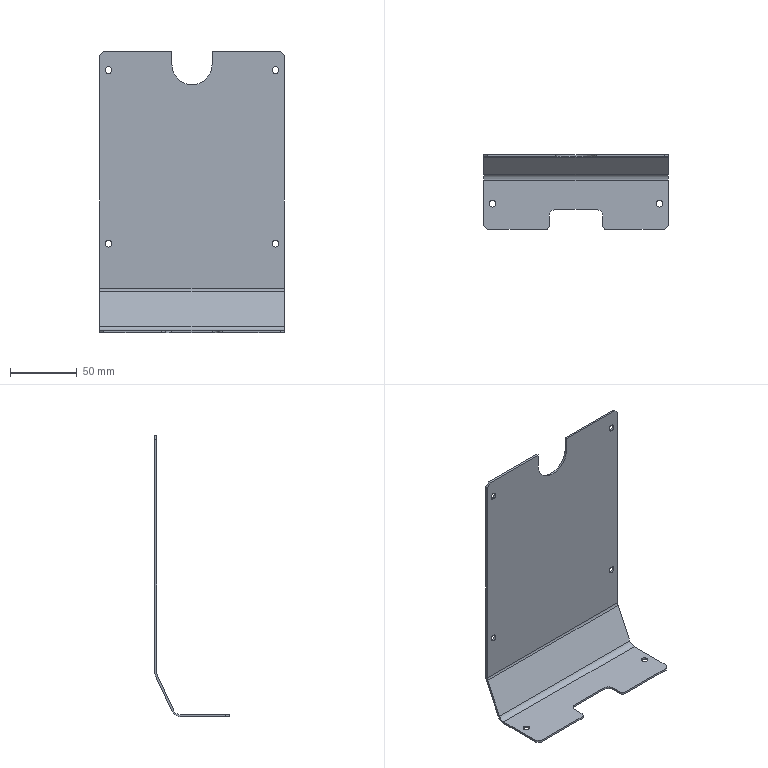Part | SolidWorks | features BaseBody 1 | 1 solid | 42 faces | box 138 x 55.773 x 210.513 mm | volume 50226 mm3 | cylinder 21 | plane 21 | commonest cylinder face diameters 5 x12 10 x4 6 x2 13 x2 30 x1
STEP:
#1=CARTESIAN_POINT('',(62.5,-33.973,-119.763));
#2=VERTEX_POINT('',#1);
#3=CARTESIAN_POINT('',(62.5,-38.973,-119.763));
#4=VERTEX_POINT('',#3);
#5=CARTESIAN_POINT('',(62.5,-36.473,-119.763));
#6=DIRECTION('',(0.,0.,1.));
#7=DIRECTION('',(0.,-1.,0.));
#8=AXIS2_PLACEMENT_3D('',#5,#6,#7);
#9=CIRCLE('',#8,2.5);
#10=EDGE_CURVE('',#2,#4,#9,.T.);
#11=ORIENTED_EDGE('',*,*,#10,.T.);
#12=CARTESIAN_POINT('',(62.5,-38.973,-121.263));
#13=VERTEX_POINT('',#12);
#14=CARTESIAN_POINT('',(62.5,-38.973,-121.263));
#15=DIRECTION('',(0.,0.,-1.));
#16=VECTOR('',#15,1000.);
#17=LINE('',#14,#16);
#18=EDGE_CURVE('',#4,#13,#17,.T.);
#19=ORIENTED_EDGE('',*,*,#18,.T.);
#20=CARTESIAN_POINT('',(62.5,-33.973,-121.263));
#21=VERTEX_POINT('',#20);
#22=CARTESIAN_POINT('',(62.5,-36.473,-121.263));
#23=DIRECTION('',(0.,0.,-1.));
#24=DIRECTION('',(0.,1.,0.));
#25=AXIS2_PLACEMENT_3D('',#22,#23,#24);
#26=CIRCLE('',#25,2.5);
#27=EDGE_CURVE('',#13,#21,#26,.T.);
#28=ORIENTED_EDGE('',*,*,#27,.T.);
#29=CARTESIAN_POINT('',(62.5,-33.973,-121.263));
#30=DIRECTION('',(0.,0.,-1.));
#31=VECTOR('',#30,1000.);
#32=LINE('',#29,#31);
#33=EDGE_CURVE('',#2,#21,#32,.T.);
#34=ORIENTED_EDGE('',*,*,#33,.F.);
#35=EDGE_LOOP('',(#11,#19,#28,#34));
#36=FACE_OUTER_BOUND('',#35,.T.);
#37=CARTESIAN_POINT('',(62.5,-36.473,-121.263));
#38=DIRECTION('',(0.,0.,-1.));
#39=DIRECTION('',(0.,1.,0.));
#40=AXIS2_PLACEMENT_3D('',#37,#38,#39);
#41=CYLINDRICAL_SURFACE('',#40,2.5);
#42=ADVANCED_FACE('',(#36),#41,.F.);
#43=CARTESIAN_POINT('',(-62.5,-33.973,-119.763));
#44=VERTEX_POINT('',#43);
#45=CARTESIAN_POINT('',(-62.5,-38.973,-119.763));
#46=VERTEX_POINT('',#45);
#47=CARTESIAN_POINT('',(-62.5,-36.473,-119.763));
#48=DIRECTION('',(0.,0.,1.));
#49=DIRECTION('',(0.,-1.,0.));
#50=AXIS2_PLACEMENT_3D('',#47,#48,#49);
#51=CIRCLE('',#50,2.5);
#52=EDGE_CURVE('',#44,#46,#51,.T.);
#53=ORIENTED_EDGE('',*,*,#52,.T.);
#54=CARTESIAN_POINT('',(-62.5,-38.973,-121.263));
#55=VERTEX_POINT('',#54);
#56=CARTESIAN_POINT('',(-62.5,-38.973,-121.263));
#57=DIRECTION('',(0.,0.,-1.));
#58=VECTOR('',#57,1000.);
#59=LINE('',#56,#58);
#60=EDGE_CURVE('',#46,#55,#59,.T.);
#61=ORIENTED_EDGE('',*,*,#60,.T.);
#62=CARTESIAN_POINT('',(-62.5,-33.973,-121.263));
#63=VERTEX_POINT('',#62);
#64=CARTESIAN_POINT('',(-62.5,-36.473,-121.263));
#65=DIRECTION('',(0.,0.,-1.));
#66=DIRECTION('',(0.,1.,0.));
#67=AXIS2_PLACEMENT_3D('',#64,#65,#66);
#68=CIRCLE('',#67,2.5);
#69=EDGE_CURVE('',#55,#63,#68,.T.);
#70=ORIENTED_EDGE('',*,*,#69,.T.);
#71=CARTESIAN_POINT('',(-62.5,-33.973,-121.263));
#72=DIRECTION('',(0.,0.,-1.));
#73=VECTOR('',#72,1000.);
#74=LINE('',#71,#73);
#75=EDGE_CURVE('',#44,#63,#74,.T.);
#76=ORIENTED_EDGE('',*,*,#75,.F.);
#77=EDGE_LOOP('',(#53,#61,#70,#76));
#78=FACE_OUTER_BOUND('',#77,.T.);
#79=CARTESIAN_POINT('',(-62.5,-36.473,-121.263));
#80=DIRECTION('',(0.,0.,-1.));
#81=DIRECTION('',(0.,1.,0.));
#82=AXIS2_PLACEMENT_3D('',#79,#80,#81);
#83=CYLINDRICAL_SURFACE('',#82,2.5);
#84=ADVANCED_FACE('',(#78),#83,.F.);
#85=CARTESIAN_POINT('',(62.5,-1.5,-57.25));
#86=VERTEX_POINT('',#85);
#87=CARTESIAN_POINT('',(62.5,-1.5,-52.25));
#88=VERTEX_POINT('',#87);
#89=CARTESIAN_POINT('',(62.5,-1.5,-54.75));
#90=DIRECTION('',(0.,1.,0.));
#91=DIRECTION('',(0.,0.,1.));
#92=AXIS2_PLACEMENT_3D('',#89,#90,#91);
#93=CIRCLE('',#92,2.5);
#94=EDGE_CURVE('',#86,#88,#93,.T.);
#95=ORIENTED_EDGE('',*,*,#94,.F.);
#96=CARTESIAN_POINT('',(62.5,0.,-57.25));
#97=VERTEX_POINT('',#96);
#98=CARTESIAN_POINT('',(62.5,0.,-57.25));
#99=DIRECTION('',(0.,1.,0.));
#100=VECTOR('',#99,1000.);
#101=LINE('',#98,#100);
#102=EDGE_CURVE('',#86,#97,#101,.T.);
#103=ORIENTED_EDGE('',*,*,#102,.T.);
#104=CARTESIAN_POINT('',(62.5,0.,-52.25));
#105=VERTEX_POINT('',#104);
#106=CARTESIAN_POINT('',(62.5,0.,-54.75));
#107=DIRECTION('',(0.,1.,0.));
#108=DIRECTION('',(0.,0.,1.));
#109=AXIS2_PLACEMENT_3D('',#106,#107,#108);
#110=CIRCLE('',#109,2.5);
#111=EDGE_CURVE('',#97,#105,#110,.T.);
#112=ORIENTED_EDGE('',*,*,#111,.T.);
#113=CARTESIAN_POINT('',(62.5,0.,-52.25));
#114=DIRECTION('',(0.,1.,0.));
#115=VECTOR('',#114,1000.);
#116=LINE('',#113,#115);
#117=EDGE_CURVE('',#88,#105,#116,.T.);
#118=ORIENTED_EDGE('',*,*,#117,.F.);
#119=EDGE_LOOP('',(#95,#103,#112,#118));
#120=FACE_OUTER_BOUND('',#119,.T.);
#121=CARTESIAN_POINT('',(62.5,0.,-54.75));
#122=DIRECTION('',(0.,1.,0.));
#123=DIRECTION('',(0.,0.,1.));
#124=AXIS2_PLACEMENT_3D('',#121,#122,#123);
#125=CYLINDRICAL_SURFACE('',#124,2.5);
#126=ADVANCED_FACE('',(#120),#125,.F.);
#127=CARTESIAN_POINT('',(-62.5,-1.5,-57.25));
#128=VERTEX_POINT('',#127);
#129=CARTESIAN_POINT('',(-62.5,-1.5,-52.25));
#130=VERTEX_POINT('',#129);
#131=CARTESIAN_POINT('',(-62.5,-1.5,-54.75));
#132=DIRECTION('',(0.,1.,0.));
#133=DIRECTION('',(0.,0.,1.));
#134=AXIS2_PLACEMENT_3D('',#131,#132,#133);
#135=CIRCLE('',#134,2.5);
#136=EDGE_CURVE('',#128,#130,#135,.T.);
#137=ORIENTED_EDGE('',*,*,#136,.F.);
#138=CARTESIAN_POINT('',(-62.5,0.,-57.25));
#139=VERTEX_POINT('',#138);
#140=CARTESIAN_POINT('',(-62.5,0.,-57.25));
#141=DIRECTION('',(0.,1.,0.));
#142=VECTOR('',#141,1000.);
#143=LINE('',#140,#142);
#144=EDGE_CURVE('',#128,#139,#143,.T.);
#145=ORIENTED_EDGE('',*,*,#144,.T.);
#146=CARTESIAN_POINT('',(-62.5,0.,-52.25));
#147=VERTEX_POINT('',#146);
#148=CARTESIAN_POINT('',(-62.5,0.,-54.75));
#149=DIRECTION('',(0.,1.,0.));
#150=DIRECTION('',(0.,0.,1.));
#151=AXIS2_PLACEMENT_3D('',#148,#149,#150);
#152=CIRCLE('',#151,2.5);
#153=EDGE_CURVE('',#139,#147,#152,.T.);
#154=ORIENTED_EDGE('',*,*,#153,.T.);
#155=CARTESIAN_POINT('',(-62.5,0.,-52.25));
#156=DIRECTION('',(0.,1.,0.));
#157=VECTOR('',#156,1000.);
#158=LINE('',#155,#157);
#159=EDGE_CURVE('',#130,#147,#158,.T.);
#160=ORIENTED_EDGE('',*,*,#159,.F.);
#161=EDGE_LOOP('',(#137,#145,#154,#160));
#162=FACE_OUTER_BOUND('',#161,.T.);
#163=CARTESIAN_POINT('',(-62.5,0.,-54.75));
#164=DIRECTION('',(0.,1.,0.));
#165=DIRECTION('',(0.,0.,1.));
#166=AXIS2_PLACEMENT_3D('',#163,#164,#165);
#167=CYLINDRICAL_SURFACE('',#166,2.5);
#168=ADVANCED_FACE('',(#162),#167,.F.);
#169=CARTESIAN_POINT('',(-62.5,-1.5,72.75));
#170=VERTEX_POINT('',#169);
#171=CARTESIAN_POINT('',(-62.5,-1.5,77.75));
#172=VERTEX_POINT('',#171);
#173=CARTESIAN_POINT('',(-62.5,-1.5,75.25));
#174=DIRECTION('',(0.,1.,0.));
#175=DIRECTION('',(0.,0.,1.));
#176=AXIS2_PLACEMENT_3D('',#173,#174,#175);
#177=CIRCLE('',#176,2.5);
#178=EDGE_CURVE('',#170,#172,#177,.T.);
#179=ORIENTED_EDGE('',*,*,#178,.F.);
#180=CARTESIAN_POINT('',(-62.5,0.,72.75));
#181=VERTEX_POINT('',#180);
#182=CARTESIAN_POINT('',(-62.5,0.,72.75));
#183=DIRECTION('',(0.,1.,0.));
#184=VECTOR('',#183,1000.);
#185=LINE('',#182,#184);
#186=EDGE_CURVE('',#170,#181,#185,.T.);
#187=ORIENTED_EDGE('',*,*,#186,.T.);
#188=CARTESIAN_POINT('',(-62.5,0.,77.75));
#189=VERTEX_POINT('',#188);
#190=CARTESIAN_POINT('',(-62.5,0.,75.25));
#191=DIRECTION('',(0.,1.,0.));
#192=DIRECTION('',(0.,0.,1.));
#193=AXIS2_PLACEMENT_3D('',#190,#191,#192);
#194=CIRCLE('',#193,2.5);
#195=EDGE_CURVE('',#181,#189,#194,.T.);
#196=ORIENTED_EDGE('',*,*,#195,.T.);
#197=CARTESIAN_POINT('',(-62.5,0.,77.75));
#198=DIRECTION('',(0.,1.,0.));
#199=VECTOR('',#198,1000.);
#200=LINE('',#197,#199);
#201=EDGE_CURVE('',#172,#189,#200,.T.);
#202=ORIENTED_EDGE('',*,*,#201,.F.);
#203=EDGE_LOOP('',(#179,#187,#196,#202));
#204=FACE_OUTER_BOUND('',#203,.T.);
#205=CARTESIAN_POINT('',(-62.5,0.,75.25));
#206=DIRECTION('',(0.,1.,0.));
#207=DIRECTION('',(0.,0.,1.));
#208=AXIS2_PLACEMENT_3D('',#205,#206,#207);
#209=CYLINDRICAL_SURFACE('',#208,2.5);
#210=ADVANCED_FACE('',(#204),#209,.F.);
#211=CARTESIAN_POINT('',(62.5,-1.5,72.75));
#212=VERTEX_POINT('',#211);
#213=CARTESIAN_POINT('',(62.5,-1.5,77.75));
#214=VERTEX_POINT('',#213);
#215=CARTESIAN_POINT('',(62.5,-1.5,75.25));
#216=DIRECTION('',(0.,1.,0.));
#217=DIRECTION('',(0.,0.,1.));
#218=AXIS2_PLACEMENT_3D('',#215,#216,#217);
#219=CIRCLE('',#218,2.5);
#220=EDGE_CURVE('',#212,#214,#219,.T.);
#221=ORIENTED_EDGE('',*,*,#220,.F.);
#222=CARTESIAN_POINT('',(62.5,0.,72.75));
#223=VERTEX_POINT('',#222);
#224=CARTESIAN_POINT('',(62.5,0.,72.75));
#225=DIRECTION('',(0.,1.,0.));
#226=VECTOR('',#225,1000.);
#227=LINE('',#224,#226);
#228=EDGE_CURVE('',#212,#223,#227,.T.);
#229=ORIENTED_EDGE('',*,*,#228,.T.);
#230=CARTESIAN_POINT('',(62.5,0.,77.75));
#231=VERTEX_POINT('',#230);
#232=CARTESIAN_POINT('',(62.5,0.,75.25));
#233=DIRECTION('',(0.,1.,0.));
#234=DIRECTION('',(0.,0.,1.));
#235=AXIS2_PLACEMENT_3D('',#232,#233,#234);
#236=CIRCLE('',#235,2.5);
#237=EDGE_CURVE('',#223,#231,#236,.T.);
#238=ORIENTED_EDGE('',*,*,#237,.T.);
#239=CARTESIAN_POINT('',(62.5,0.,77.75));
#240=DIRECTION('',(0.,1.,0.));
#241=VECTOR('',#240,1000.);
#242=LINE('',#239,#241);
#243=EDGE_CURVE('',#214,#231,#242,.T.);
#244=ORIENTED_EDGE('',*,*,#243,.F.);
#245=EDGE_LOOP('',(#221,#229,#238,#244));
#246=FACE_OUTER_BOUND('',#245,.T.);
#247=CARTESIAN_POINT('',(62.5,0.,75.25));
#248=DIRECTION('',(0.,1.,0.));
#249=DIRECTION('',(0.,0.,1.));
#250=AXIS2_PLACEMENT_3D('',#247,#248,#249);
#251=CYLINDRICAL_SURFACE('',#250,2.5);
#252=ADVANCED_FACE('',(#246),#251,.F.);
#253=CARTESIAN_POINT('',(-15.,-1.5,89.25));
#254=VERTEX_POINT('',#253);
#255=CARTESIAN_POINT('',(-15.,-1.5,79.25));
#256=VERTEX_POINT('',#255);
#257=CARTESIAN_POINT('',(-15.,-1.5,79.25));
#258=DIRECTION('',(0.,0.,-1.));
#259=VECTOR('',#258,1000.);
#260=LINE('',#257,#259);
#261=EDGE_CURVE('',#254,#256,#260,.T.);
#262=ORIENTED_EDGE('',*,*,#261,.T.);
#263=CARTESIAN_POINT('',(-15.,0.,79.25));
#264=VERTEX_POINT('',#263);
#265=CARTESIAN_POINT('',(-15.,-55.774,79.25));
#266=DIRECTION('',(0.,1.,0.));
#267=VECTOR('',#266,1000.);
#268=LINE('',#265,#267);
#269=EDGE_CURVE('',#256,#264,#268,.T.);
#270=ORIENTED_EDGE('',*,*,#269,.T.);
#271=CARTESIAN_POINT('',(-15.,0.,89.25));
#272=VERTEX_POINT('',#271);
#273=CARTESIAN_POINT('',(-15.,0.,79.25));
#274=DIRECTION('',(0.,0.,1.));
#275=VECTOR('',#274,1000.);
#276=LINE('',#273,#275);
#277=EDGE_CURVE('',#264,#272,#276,.T.);
#278=ORIENTED_EDGE('',*,*,#277,.T.);
#279=CARTESIAN_POINT('',(-15.,-55.774,89.25));
#280=DIRECTION('',(0.,1.,0.));
#281=VECTOR('',#280,1000.);
#282=LINE('',#279,#281);
#283=EDGE_CURVE('',#254,#272,#282,.T.);
#284=ORIENTED_EDGE('',*,*,#283,.F.);
#285=EDGE_LOOP('',(#262,#270,#278,#284));
#286=FACE_OUTER_BOUND('',#285,.T.);
#287=CARTESIAN_POINT('',(-15.,-55.774,79.25));
#288=DIRECTION('',(-1.,0.,0.));
#289=DIRECTION('',(0.,1.,0.));
#290=AXIS2_PLACEMENT_3D('',#287,#288,#289);
#291=PLANE('',#290);
#292=ADVANCED_FACE('',(#286),#291,.F.);
#293=CARTESIAN_POINT('',(15.,-1.5,79.25));
#294=VERTEX_POINT('',#293);
#295=CARTESIAN_POINT('',(15.,-1.5,89.25));
#296=VERTEX_POINT('',#295);
#297=CARTESIAN_POINT('',(15.,-1.5,79.25));
#298=DIRECTION('',(0.,0.,1.));
#299=VECTOR('',#298,1000.);
#300=LINE('',#297,#299);
#301=EDGE_CURVE('',#294,#296,#300,.T.);
#302=ORIENTED_EDGE('',*,*,#301,.T.);
#303=CARTESIAN_POINT('',(15.,0.,89.25));
#304=VERTEX_POINT('',#303);
#305=CARTESIAN_POINT('',(15.,-55.774,89.25));
#306=DIRECTION('',(0.,-1.,0.));
#307=VECTOR('',#306,1000.);
#308=LINE('',#305,#307);
#309=EDGE_CURVE('',#304,#296,#308,.T.);
#310=ORIENTED_EDGE('',*,*,#309,.F.);
#311=CARTESIAN_POINT('',(15.,0.,79.25));
#312=VERTEX_POINT('',#311);
#313=CARTESIAN_POINT('',(15.,0.,79.25));
#314=DIRECTION('',(0.,0.,-1.));
#315=VECTOR('',#314,1000.);
#316=LINE('',#313,#315);
#317=EDGE_CURVE('',#304,#312,#316,.T.);
#318=ORIENTED_EDGE('',*,*,#317,.T.);
#319=CARTESIAN_POINT('',(15.,-55.774,79.25));
#320=DIRECTION('',(0.,1.,0.));
#321=VECTOR('',#320,1000.);
#322=LINE('',#319,#321);
#323=EDGE_CURVE('',#294,#312,#322,.T.);
#324=ORIENTED_EDGE('',*,*,#323,.F.);
#325=EDGE_LOOP('',(#302,#310,#318,#324));
#326=FACE_OUTER_BOUND('',#325,.T.);
#327=CARTESIAN_POINT('',(15.,-55.774,79.25));
#328=DIRECTION('',(1.,0.,0.));
#329=DIRECTION('',(0.,0.,-1.));
#330=AXIS2_PLACEMENT_3D('',#327,#328,#329);
#331=PLANE('',#330);
#332=ADVANCED_FACE('',(#326),#331,.F.);
#333=CARTESIAN_POINT('',(0.,-1.5,79.25));
#334=DIRECTION('',(0.,-1.,0.));
#335=DIRECTION('',(0.,0.,1.));
#336=AXIS2_PLACEMENT_3D('',#333,#334,#335);
#337=CIRCLE('',#336,15.);
#338=EDGE_CURVE('',#256,#294,#337,.T.);
#339=ORIENTED_EDGE('',*,*,#338,.T.);
#340=ORIENTED_EDGE('',*,*,#323,.T.);
#341=CARTESIAN_POINT('',(0.,0.,79.25));
#342=DIRECTION('',(0.,1.,0.));
#343=DIRECTION('',(0.,0.,1.));
#344=AXIS2_PLACEMENT_3D('',#341,#342,#343);
#345=CIRCLE('',#344,15.);
#346=EDGE_CURVE('',#312,#264,#345,.T.);
#347=ORIENTED_EDGE('',*,*,#346,.T.);
#348=ORIENTED_EDGE('',*,*,#269,.F.);
#349=EDGE_LOOP('',(#339,#340,#347,#348));
#350=FACE_OUTER_BOUND('',#349,.T.);
#351=CARTESIAN_POINT('',(0.,-55.774,79.25));
#352=DIRECTION('',(0.,1.,0.));
#353=DIRECTION('',(0.,0.,1.));
#354=AXIS2_PLACEMENT_3D('',#351,#352,#353);
#355=CYLINDRICAL_SURFACE('',#354,15.);
#356=ADVANCED_FACE('',(#350),#355,.F.);
#357=CARTESIAN_POINT('',(20.,-52.773,-119.763));
#358=VERTEX_POINT('',#357);
#359=CARTESIAN_POINT('',(23.,-55.773,-119.763));
#360=VERTEX_POINT('',#359);
#361=CARTESIAN_POINT('',(23.,-52.773,-119.763));
#362=DIRECTION('',(0.,0.,1.));
#363=DIRECTION('',(0.,-1.,0.));
#364=AXIS2_PLACEMENT_3D('',#361,#362,#363);
#365=CIRCLE('',#364,3.);
#366=EDGE_CURVE('',#358,#360,#365,.T.);
#367=ORIENTED_EDGE('',*,*,#366,.F.);
#368=CARTESIAN_POINT('',(20.,-52.773,-121.263));
#369=VERTEX_POINT('',#368);
#370=CARTESIAN_POINT('',(20.,-52.773,89.251));
#371=DIRECTION('',(0.,0.,1.));
#372=VECTOR('',#371,1000.);
#373=LINE('',#370,#372);
#374=EDGE_CURVE('',#369,#358,#373,.T.);
#375=ORIENTED_EDGE('',*,*,#374,.F.);
#376=CARTESIAN_POINT('',(23.,-55.773,-121.263));
#377=VERTEX_POINT('',#376);
#378=CARTESIAN_POINT('',(23.,-52.773,-121.263));
#379=DIRECTION('',(0.,0.,-1.));
#380=DIRECTION('',(0.,-1.,0.));
#381=AXIS2_PLACEMENT_3D('',#378,#379,#380);
#382=CIRCLE('',#381,3.);
#383=EDGE_CURVE('',#377,#369,#382,.T.);
#384=ORIENTED_EDGE('',*,*,#383,.F.);
#385=CARTESIAN_POINT('',(23.,-55.773,-121.263));
#386=DIRECTION('',(0.,0.,-1.));
#387=VECTOR('',#386,1000.);
#388=LINE('',#385,#387);
#389=EDGE_CURVE('',#360,#377,#388,.T.);
#390=ORIENTED_EDGE('',*,*,#389,.F.);
#391=EDGE_LOOP('',(#367,#375,#384,#390));
#392=FACE_OUTER_BOUND('',#391,.T.);
#393=CARTESIAN_POINT('',(23.,-52.773,-121.263));
#394=DIRECTION('',(0.,0.,-1.));
#395=DIRECTION('',(0.,1.,0.));
#396=AXIS2_PLACEMENT_3D('',#393,#394,#395);
#397=CYLINDRICAL_SURFACE('',#396,3.);
#398=ADVANCED_FACE('',(#392),#397,.T.);
#399=CARTESIAN_POINT('',(-23.,-55.773,-119.763));
#400=VERTEX_POINT('',#399);
#401=CARTESIAN_POINT('',(-20.,-52.773,-119.763));
#402=VERTEX_POINT('',#401);
#403=CARTESIAN_POINT('',(-23.,-52.773,-119.763));
#404=DIRECTION('',(0.,0.,1.));
#405=DIRECTION('',(0.,-1.,0.));
#406=AXIS2_PLACEMENT_3D('',#403,#404,#405);
#407=CIRCLE('',#406,3.);
#408=EDGE_CURVE('',#400,#402,#407,.T.);
#409=ORIENTED_EDGE('',*,*,#408,.F.);
#410=CARTESIAN_POINT('',(-23.,-55.773,-121.263));
#411=VERTEX_POINT('',#410);
#412=CARTESIAN_POINT('',(-23.,-55.773,-121.263));
#413=DIRECTION('',(0.,0.,1.));
#414=VECTOR('',#413,1000.);
#415=LINE('',#412,#414);
#416=EDGE_CURVE('',#411,#400,#415,.T.);
#417=ORIENTED_EDGE('',*,*,#416,.F.);
#418=CARTESIAN_POINT('',(-20.,-52.773,-121.263));
#419=VERTEX_POINT('',#418);
#420=CARTESIAN_POINT('',(-23.,-52.773,-121.263));
#421=DIRECTION('',(0.,0.,-1.));
#422=DIRECTION('',(0.,-1.,0.));
#423=AXIS2_PLACEMENT_3D('',#420,#421,#422);
#424=CIRCLE('',#423,3.);
#425=EDGE_CURVE('',#419,#411,#424,.T.);
#426=ORIENTED_EDGE('',*,*,#425,.F.);
#427=CARTESIAN_POINT('',(-20.,-52.773,89.251));
#428=DIRECTION('',(0.,0.,-1.));
#429=VECTOR('',#428,1000.);
#430=LINE('',#427,#429);
#431=EDGE_CURVE('',#402,#419,#430,.T.);
#432=ORIENTED_EDGE('',*,*,#431,.F.);
#433=EDGE_LOOP('',(#409,#417,#426,#432));
#434=FACE_OUTER_BOUND('',#433,.T.);
#435=CARTESIAN_POINT('',(-23.,-52.773,89.251));
#436=DIRECTION('',(0.,0.,-1.));
#437=DIRECTION('',(0.,1.,0.));
#438=AXIS2_PLACEMENT_3D('',#435,#436,#437);
#439=CYLINDRICAL_SURFACE('',#438,3.);
#440=ADVANCED_FACE('',(#434),#439,.T.);
#441=CARTESIAN_POINT('',(15.,-40.773,-119.763));
#442=VERTEX_POINT('',#441);
#443=CARTESIAN_POINT('',(20.,-45.773,-119.763));
#444=VERTEX_POINT('',#443);
#445=CARTESIAN_POINT('',(15.,-45.773,-119.763));
#446=DIRECTION('',(0.,0.,-1.));
#447=DIRECTION('',(0.,-1.,0.));
#448=AXIS2_PLACEMENT_3D('',#445,#446,#447);
#449=CIRCLE('',#448,5.);
#450=EDGE_CURVE('',#442,#444,#449,.T.);
#451=ORIENTED_EDGE('',*,*,#450,.F.);
#452=CARTESIAN_POINT('',(15.,-40.773,-121.263));
#453=VERTEX_POINT('',#452);
#454=CARTESIAN_POINT('',(15.,-40.773,-119.763));
#455=DIRECTION('',(0.,0.,1.));
#456=VECTOR('',#455,1000.);
#457=LINE('',#454,#456);
#458=EDGE_CURVE('',#453,#442,#457,.T.);
#459=ORIENTED_EDGE('',*,*,#458,.F.);
#460=CARTESIAN_POINT('',(20.,-45.773,-121.263));
#461=VERTEX_POINT('',#460);
#462=CARTESIAN_POINT('',(15.,-45.773,-121.263));
#463=DIRECTION('',(0.,0.,1.));
#464=DIRECTION('',(0.,-1.,0.));
#465=AXIS2_PLACEMENT_3D('',#462,#463,#464);
#466=CIRCLE('',#465,5.);
#467=EDGE_CURVE('',#461,#453,#466,.T.);
#468=ORIENTED_EDGE('',*,*,#467,.F.);
#469=CARTESIAN_POINT('',(20.,-45.773,-121.263));
#470=DIRECTION('',(0.,0.,-1.));
#471=VECTOR('',#470,1000.);
#472=LINE('',#469,#471);
#473=EDGE_CURVE('',#444,#461,#472,.T.);
#474=ORIENTED_EDGE('',*,*,#473,.F.);
#475=EDGE_LOOP('',(#451,#459,#468,#474));
#476=FACE_OUTER_BOUND('',#475,.T.);
#477=CARTESIAN_POINT('',(15.,-45.773,89.251));
#478=DIRECTION('',(0.,0.,1.));
#479=DIRECTION('',(0.,-1.,0.));
#480=AXIS2_PLACEMENT_3D('',#477,#478,#479);
#481=CYLINDRICAL_SURFACE('',#480,5.);
#482=ADVANCED_FACE('',(#476),#481,.F.);
#483=CARTESIAN_POINT('',(-20.,-45.773,-119.763));
#484=VERTEX_POINT('',#483);
#485=CARTESIAN_POINT('',(-15.,-40.773,-119.763));
#486=VERTEX_POINT('',#485);
#487=CARTESIAN_POINT('',(-15.,-45.773,-119.763));
#488=DIRECTION('',(0.,0.,-1.));
#489=DIRECTION('',(0.,-1.,0.));
#490=AXIS2_PLACEMENT_3D('',#487,#488,#489);
#491=CIRCLE('',#490,5.);
#492=EDGE_CURVE('',#484,#486,#491,.T.);
#493=ORIENTED_EDGE('',*,*,#492,.F.);
#494=CARTESIAN_POINT('',(-20.,-45.773,-121.263));
#495=VERTEX_POINT('',#494);
#496=CARTESIAN_POINT('',(-20.,-45.773,-119.763));
#497=DIRECTION('',(0.,0.,1.));
#498=VECTOR('',#497,1000.);
#499=LINE('',#496,#498);
#500=EDGE_CURVE('',#495,#484,#499,.T.);
#501=ORIENTED_EDGE('',*,*,#500,.F.);
#502=CARTESIAN_POINT('',(-15.,-40.773,-121.263));
#503=VERTEX_POINT('',#502);
#504=CARTESIAN_POINT('',(-15.,-45.773,-121.263));
#505=DIRECTION('',(0.,0.,1.));
#506=DIRECTION('',(0.,-1.,0.));
#507=AXIS2_PLACEMENT_3D('',#504,#505,#506);
#508=CIRCLE('',#507,5.);
#509=EDGE_CURVE('',#503,#495,#508,.T.);
#510=ORIENTED_EDGE('',*,*,#509,.F.);
#511=CARTESIAN_POINT('',(-15.,-40.773,-121.263));
#512=DIRECTION('',(0.,0.,-1.));
#513=VECTOR('',#512,1000.);
#514=LINE('',#511,#513);
#515=EDGE_CURVE('',#486,#503,#514,.T.);
#516=ORIENTED_EDGE('',*,*,#515,.F.);
#517=EDGE_LOOP('',(#493,#501,#510,#516));
#518=FACE_OUTER_BOUND('',#517,.T.);
#519=CARTESIAN_POINT('',(-15.,-45.773,89.251));
#520=DIRECTION('',(0.,0.,1.));
#521=DIRECTION('',(0.,-1.,0.));
#522=AXIS2_PLACEMENT_3D('',#519,#520,#521);
#523=CYLINDRICAL_SURFACE('',#522,5.);
#524=ADVANCED_FACE('',(#518),#523,.F.);
#525=CARTESIAN_POINT('',(-20.,-55.773,-119.763));
#526=DIRECTION('',(0.,1.,0.));
#527=VECTOR('',#526,1000.);
#528=LINE('',#525,#527);
#529=EDGE_CURVE('',#402,#484,#528,.T.);
#530=ORIENTED_EDGE('',*,*,#529,.F.);
#531=ORIENTED_EDGE('',*,*,#431,.T.);
#532=CARTESIAN_POINT('',(-20.,-55.773,-121.263));
#533=DIRECTION('',(0.,1.,0.));
#534=VECTOR('',#533,1000.);
#535=LINE('',#532,#534);
#536=EDGE_CURVE('',#419,#495,#535,.T.);
#537=ORIENTED_EDGE('',*,*,#536,.T.);
#538=ORIENTED_EDGE('',*,*,#500,.T.);
#539=EDGE_LOOP('',(#530,#531,#537,#538));
#540=FACE_OUTER_BOUND('',#539,.T.);
#541=CARTESIAN_POINT('',(-20.,-55.773,89.251));
#542=DIRECTION('',(-1.,0.,0.));
#543=DIRECTION('',(0.,0.,1.));
#544=AXIS2_PLACEMENT_3D('',#541,#542,#543);
#545=PLANE('',#544);
#546=ADVANCED_FACE('',(#540),#545,.F.);
#547=CARTESIAN_POINT('',(20.,-40.773,-119.763));
#548=DIRECTION('',(1.,0.,0.));
#549=VECTOR('',#548,1000.);
#550=LINE('',#547,#549);
#551=EDGE_CURVE('',#486,#442,#550,.T.);
#552=ORIENTED_EDGE('',*,*,#551,.F.);
#553=ORIENTED_EDGE('',*,*,#515,.T.);
#554=CARTESIAN_POINT('',(20.,-40.773,-121.263));
#555=DIRECTION('',(1.,0.,0.));
#556=VECTOR('',#555,1000.);
#557=LINE('',#554,#556);
#558=EDGE_CURVE('',#503,#453,#557,.T.);
#559=ORIENTED_EDGE('',*,*,#558,.T.);
#560=ORIENTED_EDGE('',*,*,#458,.T.);
#561=EDGE_LOOP('',(#552,#553,#559,#560));
#562=FACE_OUTER_BOUND('',#561,.T.);
#563=CARTESIAN_POINT('',(20.,-40.773,89.251));
#564=DIRECTION('',(0.,1.,0.));
#565=DIRECTION('',(0.,0.,-1.));
#566=AXIS2_PLACEMENT_3D('',#563,#564,#565);
#567=PLANE('',#566);
#568=ADVANCED_FACE('',(#562),#567,.F.);
#569=CARTESIAN_POINT('',(20.,-55.773,-121.263));
#570=DIRECTION('',(0.,-1.,0.));
#571=VECTOR('',#570,1000.);
#572=LINE('',#569,#571);
#573=EDGE_CURVE('',#461,#369,#572,.T.);
#574=ORIENTED_EDGE('',*,*,#573,.T.);
#575=ORIENTED_EDGE('',*,*,#374,.T.);
#576=CARTESIAN_POINT('',(20.,-55.773,-119.763));
#577=DIRECTION('',(0.,-1.,0.));
#578=VECTOR('',#577,1000.);
#579=LINE('',#576,#578);
#580=EDGE_CURVE('',#444,#358,#579,.T.);
#581=ORIENTED_EDGE('',*,*,#580,.F.);
#582=ORIENTED_EDGE('',*,*,#473,.T.);
#583=EDGE_LOOP('',(#574,#575,#581,#582));
#584=FACE_OUTER_BOUND('',#583,.T.);
#585=CARTESIAN_POINT('',(20.,-55.773,89.251));
#586=DIRECTION('',(1.,0.,0.));
#587=DIRECTION('',(0.,1.,0.));
#588=AXIS2_PLACEMENT_3D('',#585,#586,#587);
#589=PLANE('',#588);
#590=ADVANCED_FACE('',(#584),#589,.F.);
#591=CARTESIAN_POINT('',(69.,-52.773,-121.263));
#592=VERTEX_POINT('',#591);
#593=CARTESIAN_POINT('',(66.,-55.773,-121.263));
#594=VERTEX_POINT('',#593);
#595=CARTESIAN_POINT('',(66.,-55.773,-121.263));
#596=DIRECTION('',(-0.7071,-0.7071,0.));
#597=VECTOR('',#596,1000.);
#598=LINE('',#595,#597);
#599=EDGE_CURVE('',#592,#594,#598,.T.);
#600=ORIENTED_EDGE('',*,*,#599,.F.);
#601=CARTESIAN_POINT('',(69.,-52.773,-119.763));
#602=VERTEX_POINT('',#601);
#603=CARTESIAN_POINT('',(69.,-52.773,-121.263));
#604=DIRECTION('',(0.,0.,-1.));
#605=VECTOR('',#604,1000.);
#606=LINE('',#603,#605);
#607=EDGE_CURVE('',#602,#592,#606,.T.);
#608=ORIENTED_EDGE('',*,*,#607,.F.);
#609=CARTESIAN_POINT('',(66.,-55.773,-119.763));
#610=VERTEX_POINT('',#609);
#611=CARTESIAN_POINT('',(60.886,-60.886,-119.763));
#612=DIRECTION('',(0.7071,0.7071,0.));
#613=VECTOR('',#612,1000.);
#614=LINE('',#611,#613);
#615=EDGE_CURVE('',#610,#602,#614,.T.);
#616=ORIENTED_EDGE('',*,*,#615,.F.);
#617=CARTESIAN_POINT('',(66.,-55.773,-121.263));
#618=DIRECTION('',(0.,0.,1.));
#619=VECTOR('',#618,1000.);
#620=LINE('',#617,#619);
#621=EDGE_CURVE('',#594,#610,#620,.T.);
#622=ORIENTED_EDGE('',*,*,#621,.F.);
#623=EDGE_LOOP('',(#600,#608,#616,#622));
#624=FACE_OUTER_BOUND('',#623,.T.);
#625=CARTESIAN_POINT('',(66.,-55.773,-121.263));
#626=DIRECTION('',(-0.7071,0.7071,0.));
#627=DIRECTION('',(0.,0.,1.));
#628=AXIS2_PLACEMENT_3D('',#625,#626,#627);
#629=PLANE('',#628);
#630=ADVANCED_FACE('',(#624),#629,.F.);
#631=CARTESIAN_POINT('',(69.,-1.5,86.25));
#632=VERTEX_POINT('',#631);
#633=CARTESIAN_POINT('',(66.,-1.5,89.25));
#634=VERTEX_POINT('',#633);
#635=CARTESIAN_POINT('',(66.,-1.5,89.25));
#636=DIRECTION('',(-0.7071,0.,0.7071));
#637=VECTOR('',#636,1000.);
#638=LINE('',#635,#637);
#639=EDGE_CURVE('',#632,#634,#638,.T.);
#640=ORIENTED_EDGE('',*,*,#639,.F.);
#641=CARTESIAN_POINT('',(69.,0.,86.25));
#642=VERTEX_POINT('',#641);
#643=CARTESIAN_POINT('',(69.,-1.5,86.25));
#644=DIRECTION('',(0.,-1.,0.));
#645=VECTOR('',#644,1000.);
#646=LINE('',#643,#645);
#647=EDGE_CURVE('',#642,#632,#646,.T.);
#648=ORIENTED_EDGE('',*,*,#647,.F.);
#649=CARTESIAN_POINT('',(66.,0.,89.25));
#650=VERTEX_POINT('',#649);
#651=CARTESIAN_POINT('',(77.625,0.,77.625));
#652=DIRECTION('',(0.7071,0.,-0.7071));
#653=VECTOR('',#652,1000.);
#654=LINE('',#651,#653);
#655=EDGE_CURVE('',#650,#642,#654,.T.);
#656=ORIENTED_EDGE('',*,*,#655,.F.);
#657=CARTESIAN_POINT('',(66.,-1.5,89.25));
#658=DIRECTION('',(0.,1.,0.));
#659=VECTOR('',#658,1000.);
#660=LINE('',#657,#659);
#661=EDGE_CURVE('',#634,#650,#660,.T.);
#662=ORIENTED_EDGE('',*,*,#661,.F.);
#663=EDGE_LOOP('',(#640,#648,#656,#662));
#664=FACE_OUTER_BOUND('',#663,.T.);
#665=CARTESIAN_POINT('',(66.,-1.5,89.25));
#666=DIRECTION('',(-0.7071,0.,-0.7071));
#667=DIRECTION('',(-0.7071,0.,0.7071));
#668=AXIS2_PLACEMENT_3D('',#665,#666,#667);
#669=PLANE('',#668);
#670=ADVANCED_FACE('',(#664),#669,.F.);
#671=CARTESIAN_POINT('',(-66.,-1.5,89.25));
#672=VERTEX_POINT('',#671);
#673=CARTESIAN_POINT('',(-69.,-1.5,86.25));
#674=VERTEX_POINT('',#673);
#675=CARTESIAN_POINT('',(-69.,-1.5,86.25));
#676=DIRECTION('',(-0.7071,0.,-0.7071));
#677=VECTOR('',#676,1000.);
#678=LINE('',#675,#677);
#679=EDGE_CURVE('',#672,#674,#678,.T.);
#680=ORIENTED_EDGE('',*,*,#679,.F.);
#681=CARTESIAN_POINT('',(-66.,0.,89.25));
#682=VERTEX_POINT('',#681);
#683=CARTESIAN_POINT('',(-66.,-1.5,89.25));
#684=DIRECTION('',(0.,-1.,0.));
#685=VECTOR('',#684,1000.);
#686=LINE('',#683,#685);
#687=EDGE_CURVE('',#682,#672,#686,.T.);
#688=ORIENTED_EDGE('',*,*,#687,.F.);
#689=CARTESIAN_POINT('',(-69.,0.,86.25));
#690=VERTEX_POINT('',#689);
#691=CARTESIAN_POINT('',(-77.625,0.,77.625));
#692=DIRECTION('',(0.7071,0.,0.7071));
#693=VECTOR('',#692,1000.);
#694=LINE('',#691,#693);
#695=EDGE_CURVE('',#690,#682,#694,.T.);
#696=ORIENTED_EDGE('',*,*,#695,.F.);
#697=CARTESIAN_POINT('',(-69.,-1.5,86.25));
#698=DIRECTION('',(0.,1.,0.));
#699=VECTOR('',#698,1000.);
#700=LINE('',#697,#699);
#701=EDGE_CURVE('',#674,#690,#700,.T.);
#702=ORIENTED_EDGE('',*,*,#701,.F.);
#703=EDGE_LOOP('',(#680,#688,#696,#702));
#704=FACE_OUTER_BOUND('',#703,.T.);
#705=CARTESIAN_POINT('',(-69.,-1.5,86.25));
#706=DIRECTION('',(0.7071,0.,-0.7071));
#707=DIRECTION('',(0.,-1.,0.));
#708=AXIS2_PLACEMENT_3D('',#705,#706,#707);
#709=PLANE('',#708);
#710=ADVANCED_FACE('',(#704),#709,.F.);
#711=CARTESIAN_POINT('',(-66.,-55.773,-121.263));
#712=VERTEX_POINT('',#711);
#713=CARTESIAN_POINT('',(-69.,-52.773,-121.263));
#714=VERTEX_POINT('',#713);
#715=CARTESIAN_POINT('',(-69.,-52.773,-121.263));
#716=DIRECTION('',(-0.7071,0.7071,0.));
#717=VECTOR('',#716,1000.);
#718=LINE('',#715,#717);
#719=EDGE_CURVE('',#712,#714,#718,.T.);
#720=ORIENTED_EDGE('',*,*,#719,.F.);
#721=CARTESIAN_POINT('',(-66.,-55.773,-119.763));
#722=VERTEX_POINT('',#721);
#723=CARTESIAN_POINT('',(-66.,-55.773,-121.263));
#724=DIRECTION('',(0.,0.,-1.));
#725=VECTOR('',#724,1000.);
#726=LINE('',#723,#725);
#727=EDGE_CURVE('',#722,#712,#726,.T.);
#728=ORIENTED_EDGE('',*,*,#727,.F.);
#729=CARTESIAN_POINT('',(-69.,-52.773,-119.763));
#730=VERTEX_POINT('',#729);
#731=CARTESIAN_POINT('',(-60.886,-60.886,-119.763));
#732=DIRECTION('',(0.7071,-0.7071,0.));
#733=VECTOR('',#732,1000.);
#734=LINE('',#731,#733);
#735=EDGE_CURVE('',#730,#722,#734,.T.);
#736=ORIENTED_EDGE('',*,*,#735,.F.);
#737=CARTESIAN_POINT('',(-69.,-52.773,-121.263));
#738=DIRECTION('',(0.,0.,1.));
#739=VECTOR('',#738,1000.);
#740=LINE('',#737,#739);
#741=EDGE_CURVE('',#714,#730,#740,.T.);
#742=ORIENTED_EDGE('',*,*,#741,.F.);
#743=EDGE_LOOP('',(#720,#728,#736,#742));
#744=FACE_OUTER_BOUND('',#743,.T.);
#745=CARTESIAN_POINT('',(-69.,-52.773,-121.263));
#746=DIRECTION('',(0.7071,0.7071,0.));
#747=DIRECTION('',(0.,0.,-1.));
#748=AXIS2_PLACEMENT_3D('',#745,#746,#747);
#749=PLANE('',#748);
#750=ADVANCED_FACE('',(#744),#749,.F.);
#751=CARTESIAN_POINT('',(-69.,-55.773,-121.263));
#752=DIRECTION('',(-1.,0.,0.));
#753=VECTOR('',#752,1000.);
#754=LINE('',#751,#753);
#755=EDGE_CURVE('',#411,#712,#754,.T.);
#756=ORIENTED_EDGE('',*,*,#755,.F.);
#757=ORIENTED_EDGE('',*,*,#416,.T.);
#758=CARTESIAN_POINT('',(-69.,-55.773,-119.763));
#759=DIRECTION('',(-1.,0.,0.));
#760=VECTOR('',#759,1000.);
#761=LINE('',#758,#760);
#762=EDGE_CURVE('',#400,#722,#761,.T.);
#763=ORIENTED_EDGE('',*,*,#762,.T.);
#764=ORIENTED_EDGE('',*,*,#727,.T.);
#765=EDGE_LOOP('',(#756,#757,#763,#764));
#766=FACE_OUTER_BOUND('',#765,.T.);
#767=CARTESIAN_POINT('',(-69.,-55.773,-121.263));
#768=DIRECTION('',(0.,1.,0.));
#769=DIRECTION('',(0.,0.,-1.));
#770=AXIS2_PLACEMENT_3D('',#767,#768,#769);
#771=PLANE('',#770);
#772=ADVANCED_FACE('',(#766),#771,.F.);
#773=ORIENTED_EDGE('',*,*,#52,.F.);
#774=CARTESIAN_POINT('',(-62.5,-36.473,-119.763));
#775=DIRECTION('',(0.,0.,1.));
#776=DIRECTION('',(0.,-1.,0.));
#777=AXIS2_PLACEMENT_3D('',#774,#775,#776);
#778=CIRCLE('',#777,2.5);
#779=EDGE_CURVE('',#46,#44,#778,.T.);
#780=ORIENTED_EDGE('',*,*,#779,.F.);
#781=EDGE_LOOP('',(#773,#780));
#782=FACE_BOUND('',#781,.T.);
#783=ORIENTED_EDGE('',*,*,#10,.F.);
#784=CARTESIAN_POINT('',(62.5,-36.473,-119.763));
#785=DIRECTION('',(0.,0.,1.));
#786=DIRECTION('',(0.,-1.,0.));
#787=AXIS2_PLACEMENT_3D('',#784,#785,#786);
#788=CIRCLE('',#787,2.5);
#789=EDGE_CURVE('',#4,#2,#788,.T.);
#790=ORIENTED_EDGE('',*,*,#789,.F.);
#791=EDGE_LOOP('',(#783,#790));
#792=FACE_BOUND('',#791,.T.);
#793=ORIENTED_EDGE('',*,*,#762,.F.);
#794=ORIENTED_EDGE('',*,*,#408,.T.);
#795=ORIENTED_EDGE('',*,*,#529,.T.);
#796=ORIENTED_EDGE('',*,*,#492,.T.);
#797=ORIENTED_EDGE('',*,*,#551,.T.);
#798=ORIENTED_EDGE('',*,*,#450,.T.);
#799=ORIENTED_EDGE('',*,*,#580,.T.);
#800=ORIENTED_EDGE('',*,*,#366,.T.);
#801=CARTESIAN_POINT('',(-69.,-55.773,-119.763));
#802=DIRECTION('',(-1.,0.,0.));
#803=VECTOR('',#802,1000.);
#804=LINE('',#801,#803);
#805=EDGE_CURVE('',#610,#360,#804,.T.);
#806=ORIENTED_EDGE('',*,*,#805,.F.);
#807=ORIENTED_EDGE('',*,*,#615,.T.);
#808=CARTESIAN_POINT('',(69.,-18.914,-119.763));
#809=VERTEX_POINT('',#808);
#810=CARTESIAN_POINT('',(69.,-55.773,-119.763));
#811=DIRECTION('',(0.,-1.,0.));
#812=VECTOR('',#811,1000.);
#813=LINE('',#810,#812);
#814=EDGE_CURVE('',#809,#602,#813,.T.);
#815=ORIENTED_EDGE('',*,*,#814,.F.);
#816=CARTESIAN_POINT('',(-69.,-18.914,-119.763));
#817=VERTEX_POINT('',#816);
#818=CARTESIAN_POINT('',(-69.,-18.914,-119.763));
#819=DIRECTION('',(1.,0.,0.));
#820=VECTOR('',#819,1000.);
#821=LINE('',#818,#820);
#822=EDGE_CURVE('',#817,#809,#821,.T.);
#823=ORIENTED_EDGE('',*,*,#822,.F.);
#824=CARTESIAN_POINT('',(-69.,-15.728,-119.763));
#825=DIRECTION('',(0.,1.,0.));
#826=VECTOR('',#825,1000.);
#827=LINE('',#824,#826);
#828=EDGE_CURVE('',#730,#817,#827,.T.);
#829=ORIENTED_EDGE('',*,*,#828,.F.);
#830=ORIENTED_EDGE('',*,*,#735,.T.);
#831=EDGE_LOOP('',(#793,#794,#795,#796,#797,#798,#799,#800,#806,#807,#815,#823,#829,#830));
#832=FACE_OUTER_BOUND('',#831,.T.);
#833=CARTESIAN_POINT('',(0.,0.,-119.763));
#834=DIRECTION('',(0.,0.,1.));
#835=DIRECTION('',(0.,-1.,0.));
#836=AXIS2_PLACEMENT_3D('',#833,#834,#835);
#837=PLANE('',#836);
#838=ADVANCED_FACE('',(#782,#792,#832),#837,.T.);
#839=CARTESIAN_POINT('',(-62.5,-36.473,-121.263));
#840=DIRECTION('',(0.,0.,-1.));
#841=DIRECTION('',(0.,1.,0.));
#842=AXIS2_PLACEMENT_3D('',#839,#840,#841);
#843=CIRCLE('',#842,2.5);
#844=EDGE_CURVE('',#63,#55,#843,.T.);
#845=ORIENTED_EDGE('',*,*,#844,.F.);
#846=ORIENTED_EDGE('',*,*,#69,.F.);
#847=EDGE_LOOP('',(#845,#846));
#848=FACE_BOUND('',#847,.T.);
#849=CARTESIAN_POINT('',(62.5,-36.473,-121.263));
#850=DIRECTION('',(0.,0.,-1.));
#851=DIRECTION('',(0.,1.,0.));
#852=AXIS2_PLACEMENT_3D('',#849,#850,#851);
#853=CIRCLE('',#852,2.5);
#854=EDGE_CURVE('',#21,#13,#853,.T.);
#855=ORIENTED_EDGE('',*,*,#854,.F.);
#856=ORIENTED_EDGE('',*,*,#27,.F.);
#857=EDGE_LOOP('',(#855,#856));
#858=FACE_BOUND('',#857,.T.);
#859=ORIENTED_EDGE('',*,*,#536,.F.);
#860=ORIENTED_EDGE('',*,*,#425,.T.);
#861=ORIENTED_EDGE('',*,*,#755,.T.);
#862=ORIENTED_EDGE('',*,*,#719,.T.);
#863=CARTESIAN_POINT('',(-69.,-18.914,-121.263));
#864=VERTEX_POINT('',#863);
#865=CARTESIAN_POINT('',(-69.,-15.728,-121.263));
#866=DIRECTION('',(0.,1.,0.));
#867=VECTOR('',#866,1000.);
#868=LINE('',#865,#867);
#869=EDGE_CURVE('',#714,#864,#868,.T.);
#870=ORIENTED_EDGE('',*,*,#869,.T.);
#871=CARTESIAN_POINT('',(69.,-18.914,-121.263));
#872=VERTEX_POINT('',#871);
#873=CARTESIAN_POINT('',(0.,-18.914,-121.263));
#874=DIRECTION('',(-1.,0.,0.));
#875=VECTOR('',#874,1000.);
#876=LINE('',#873,#875);
#877=EDGE_CURVE('',#872,#864,#876,.T.);
#878=ORIENTED_EDGE('',*,*,#877,.F.);
#879=CARTESIAN_POINT('',(69.,-55.773,-121.263));
#880=DIRECTION('',(0.,-1.,0.));
#881=VECTOR('',#880,1000.);
#882=LINE('',#879,#881);
#883=EDGE_CURVE('',#872,#592,#882,.T.);
#884=ORIENTED_EDGE('',*,*,#883,.T.);
#885=ORIENTED_EDGE('',*,*,#599,.T.);
#886=CARTESIAN_POINT('',(-69.,-55.773,-121.263));
#887=DIRECTION('',(-1.,0.,0.));
#888=VECTOR('',#887,1000.);
#889=LINE('',#886,#888);
#890=EDGE_CURVE('',#594,#377,#889,.T.);
#891=ORIENTED_EDGE('',*,*,#890,.T.);
#892=ORIENTED_EDGE('',*,*,#383,.T.);
#893=ORIENTED_EDGE('',*,*,#573,.F.);
#894=ORIENTED_EDGE('',*,*,#467,.T.);
#895=ORIENTED_EDGE('',*,*,#558,.F.);
#896=ORIENTED_EDGE('',*,*,#509,.T.);
#897=EDGE_LOOP('',(#859,#860,#861,#862,#870,#878,#884,#885,#891,#892,#893,#894,#895,#896));
#898=FACE_OUTER_BOUND('',#897,.T.);
#899=CARTESIAN_POINT('',(0.,0.,-121.263));
#900=DIRECTION('',(0.,0.,1.));
#901=DIRECTION('',(0.,-1.,0.));
#902=AXIS2_PLACEMENT_3D('',#899,#900,#901);
#903=PLANE('',#902);
#904=ADVANCED_FACE('',(#848,#858,#898),#903,.F.);
#905=CARTESIAN_POINT('',(69.,-14.382,-116.876));
#906=VERTEX_POINT('',#905);
#907=CARTESIAN_POINT('',(-69.,-14.382,-116.876));
#908=VERTEX_POINT('',#907);
#909=CARTESIAN_POINT('',(69.,-14.382,-116.876));
#910=DIRECTION('',(-1.,0.,0.));
#911=VECTOR('',#910,1000.);
#912=LINE('',#909,#911);
#913=EDGE_CURVE('',#906,#908,#912,.T.);
#914=ORIENTED_EDGE('',*,*,#913,.T.);
#915=CARTESIAN_POINT('',(-69.,-18.914,-114.763));
#916=DIRECTION('',(-1.,0.,0.));
#917=DIRECTION('',(0.,0.,-1.));
#918=AXIS2_PLACEMENT_3D('',#915,#916,#917);
#919=CIRCLE('',#918,5.);
#920=EDGE_CURVE('',#908,#817,#919,.T.);
#921=ORIENTED_EDGE('',*,*,#920,.T.);
#922=ORIENTED_EDGE('',*,*,#822,.T.);
#923=CARTESIAN_POINT('',(69.,-18.914,-114.763));
#924=DIRECTION('',(1.,0.,0.));
#925=DIRECTION('',(0.,0.,-1.));
#926=AXIS2_PLACEMENT_3D('',#923,#924,#925);
#927=CIRCLE('',#926,5.);
#928=EDGE_CURVE('',#809,#906,#927,.T.);
#929=ORIENTED_EDGE('',*,*,#928,.T.);
#930=EDGE_LOOP('',(#914,#921,#922,#929));
#931=FACE_OUTER_BOUND('',#930,.T.);
#932=CARTESIAN_POINT('',(69.,-18.914,-114.763));
#933=DIRECTION('',(1.,0.,0.));
#934=DIRECTION('',(0.,0.,-1.));
#935=AXIS2_PLACEMENT_3D('',#932,#933,#934);
#936=CYLINDRICAL_SURFACE('',#935,5.);
#937=ADVANCED_FACE('',(#931),#936,.F.);
#938=CARTESIAN_POINT('',(69.,-13.023,-117.51));
#939=VERTEX_POINT('',#938);
#940=CARTESIAN_POINT('',(-69.,-13.023,-117.51));
#941=VERTEX_POINT('',#940);
#942=CARTESIAN_POINT('',(69.,-13.023,-117.51));
#943=DIRECTION('',(-1.,0.,0.));
#944=VECTOR('',#943,1000.);
#945=LINE('',#942,#944);
#946=EDGE_CURVE('',#939,#941,#945,.T.);
#947=ORIENTED_EDGE('',*,*,#946,.F.);
#948=CARTESIAN_POINT('',(69.,-18.914,-114.763));
#949=DIRECTION('',(1.,0.,0.));
#950=DIRECTION('',(0.,0.,-1.));
#951=AXIS2_PLACEMENT_3D('',#948,#949,#950);
#952=CIRCLE('',#951,6.5);
#953=EDGE_CURVE('',#872,#939,#952,.T.);
#954=ORIENTED_EDGE('',*,*,#953,.F.);
#955=ORIENTED_EDGE('',*,*,#877,.T.);
#956=CARTESIAN_POINT('',(-69.,-18.914,-114.763));
#957=DIRECTION('',(-1.,0.,0.));
#958=DIRECTION('',(0.,0.,-1.));
#959=AXIS2_PLACEMENT_3D('',#956,#957,#958);
#960=CIRCLE('',#959,6.5);
#961=EDGE_CURVE('',#941,#864,#960,.T.);
#962=ORIENTED_EDGE('',*,*,#961,.F.);
#963=EDGE_LOOP('',(#947,#954,#955,#962));
#964=FACE_OUTER_BOUND('',#963,.T.);
#965=CARTESIAN_POINT('',(69.,-18.914,-114.763));
#966=DIRECTION('',(1.,0.,0.));
#967=DIRECTION('',(0.,0.,-1.));
#968=AXIS2_PLACEMENT_3D('',#965,#966,#967);
#969=CYLINDRICAL_SURFACE('',#968,6.5);
#970=ADVANCED_FACE('',(#964),#969,.T.);
#971=CARTESIAN_POINT('',(69.,-1.5,-88.142));
#972=VERTEX_POINT('',#971);
#973=CARTESIAN_POINT('',(-69.,-1.5,-88.142));
#974=VERTEX_POINT('',#973);
#975=CARTESIAN_POINT('',(69.,-1.5,-88.142));
#976=DIRECTION('',(-1.,0.,0.));
#977=VECTOR('',#976,1000.);
#978=LINE('',#975,#977);
#979=EDGE_CURVE('',#972,#974,#978,.T.);
#980=ORIENTED_EDGE('',*,*,#979,.T.);
#981=CARTESIAN_POINT('',(-69.,-1.968,-90.255));
#982=VERTEX_POINT('',#981);
#983=CARTESIAN_POINT('',(-69.,-6.5,-88.142));
#984=DIRECTION('',(-1.,0.,0.));
#985=DIRECTION('',(0.,0.,-1.));
#986=AXIS2_PLACEMENT_3D('',#983,#984,#985);
#987=CIRCLE('',#986,5.);
#988=EDGE_CURVE('',#974,#982,#987,.T.);
#989=ORIENTED_EDGE('',*,*,#988,.T.);
#990=CARTESIAN_POINT('',(69.,-1.968,-90.255));
#991=VERTEX_POINT('',#990);
#992=CARTESIAN_POINT('',(-69.,-1.968,-90.255));
#993=DIRECTION('',(1.,0.,0.));
#994=VECTOR('',#993,1000.);
#995=LINE('',#992,#994);
#996=EDGE_CURVE('',#982,#991,#995,.T.);
#997=ORIENTED_EDGE('',*,*,#996,.T.);
#998=CARTESIAN_POINT('',(69.,-6.5,-88.142));
#999=DIRECTION('',(1.,0.,0.));
#1000=DIRECTION('',(0.,0.,-1.));
#1001=AXIS2_PLACEMENT_3D('',#998,#999,#1000);
#1002=CIRCLE('',#1001,5.);
#1003=EDGE_CURVE('',#991,#972,#1002,.T.);
#1004=ORIENTED_EDGE('',*,*,#1003,.T.);
#1005=EDGE_LOOP('',(#980,#989,#997,#1004));
#1006=FACE_OUTER_BOUND('',#1005,.T.);
#1007=CARTESIAN_POINT('',(69.,-6.5,-88.142));
#1008=DIRECTION('',(1.,0.,0.));
#1009=DIRECTION('',(0.,0.9063,-0.4226));
#1010=AXIS2_PLACEMENT_3D('',#1007,#1008,#1009);
#1011=CYLINDRICAL_SURFACE('',#1010,5.);
#1012=ADVANCED_FACE('',(#1006),#1011,.F.);
#1013=CARTESIAN_POINT('',(69.,0.,-88.142));
#1014=VERTEX_POINT('',#1013);
#1015=CARTESIAN_POINT('',(-69.,0.,-88.142));
#1016=VERTEX_POINT('',#1015);
#1017=CARTESIAN_POINT('',(69.,0.,-88.142));
#1018=DIRECTION('',(-1.,0.,0.));
#1019=VECTOR('',#1018,1000.);
#1020=LINE('',#1017,#1019);
#1021=EDGE_CURVE('',#1014,#1016,#1020,.T.);
#1022=ORIENTED_EDGE('',*,*,#1021,.F.);
#1023=CARTESIAN_POINT('',(69.,-0.609,-90.889));
#1024=VERTEX_POINT('',#1023);
#1025=CARTESIAN_POINT('',(69.,-6.5,-88.142));
#1026=DIRECTION('',(1.,0.,0.));
#1027=DIRECTION('',(0.,0.,-1.));
#1028=AXIS2_PLACEMENT_3D('',#1025,#1026,#1027);
#1029=CIRCLE('',#1028,6.5);
#1030=EDGE_CURVE('',#1024,#1014,#1029,.T.);
#1031=ORIENTED_EDGE('',*,*,#1030,.F.);
#1032=CARTESIAN_POINT('',(-69.,-0.609,-90.889));
#1033=VERTEX_POINT('',#1032);
#1034=CARTESIAN_POINT('',(0.,-0.609,-90.889));
#1035=DIRECTION('',(-1.,0.,0.));
#1036=VECTOR('',#1035,1000.);
#1037=LINE('',#1034,#1036);
#1038=EDGE_CURVE('',#1024,#1033,#1037,.T.);
#1039=ORIENTED_EDGE('',*,*,#1038,.T.);
#1040=CARTESIAN_POINT('',(-69.,-6.5,-88.142));
#1041=DIRECTION('',(-1.,0.,0.));
#1042=DIRECTION('',(0.,0.,-1.));
#1043=AXIS2_PLACEMENT_3D('',#1040,#1041,#1042);
#1044=CIRCLE('',#1043,6.5);
#1045=EDGE_CURVE('',#1016,#1033,#1044,.T.);
#1046=ORIENTED_EDGE('',*,*,#1045,.F.);
#1047=EDGE_LOOP('',(#1022,#1031,#1039,#1046));
#1048=FACE_OUTER_BOUND('',#1047,.T.);
#1049=CARTESIAN_POINT('',(69.,-6.5,-88.142));
#1050=DIRECTION('',(1.,0.,0.));
#1051=DIRECTION('',(0.,0.9063,-0.4226));
#1052=AXIS2_PLACEMENT_3D('',#1049,#1050,#1051);
#1053=CYLINDRICAL_SURFACE('',#1052,6.5);
#1054=ADVANCED_FACE('',(#1048),#1053,.T.);
#1055=ORIENTED_EDGE('',*,*,#283,.T.);
#1056=CARTESIAN_POINT('',(-69.,0.,89.25));
#1057=DIRECTION('',(1.,0.,0.));
#1058=VECTOR('',#1057,1000.);
#1059=LINE('',#1056,#1058);
#1060=EDGE_CURVE('',#682,#272,#1059,.T.);
#1061=ORIENTED_EDGE('',*,*,#1060,.F.);
#1062=ORIENTED_EDGE('',*,*,#687,.T.);
#1063=CARTESIAN_POINT('',(-69.,-1.5,89.25));
#1064=DIRECTION('',(1.,0.,0.));
#1065=VECTOR('',#1064,1000.);
#1066=LINE('',#1063,#1065);
#1067=EDGE_CURVE('',#672,#254,#1066,.T.);
#1068=ORIENTED_EDGE('',*,*,#1067,.T.);
#1069=EDGE_LOOP('',(#1055,#1061,#1062,#1068));
#1070=FACE_OUTER_BOUND('',#1069,.T.);
#1071=CARTESIAN_POINT('',(-69.,-1.5,89.25));
#1072=DIRECTION('',(0.,0.,1.));
#1073=DIRECTION('',(1.,0.,0.));
#1074=AXIS2_PLACEMENT_3D('',#1071,#1072,#1073);
#1075=PLANE('',#1074);
#1076=ADVANCED_FACE('',(#1070),#1075,.T.);
#1077=CARTESIAN_POINT('',(62.5,0.,75.25));
#1078=DIRECTION('',(0.,1.,0.));
#1079=DIRECTION('',(0.,0.,1.));
#1080=AXIS2_PLACEMENT_3D('',#1077,#1078,#1079);
#1081=CIRCLE('',#1080,2.5);
#1082=EDGE_CURVE('',#231,#223,#1081,.T.);
#1083=ORIENTED_EDGE('',*,*,#1082,.F.);
#1084=ORIENTED_EDGE('',*,*,#237,.F.);
#1085=EDGE_LOOP('',(#1083,#1084));
#1086=FACE_BOUND('',#1085,.T.);
#1087=CARTESIAN_POINT('',(-62.5,0.,75.25));
#1088=DIRECTION('',(0.,1.,0.));
#1089=DIRECTION('',(0.,0.,1.));
#1090=AXIS2_PLACEMENT_3D('',#1087,#1088,#1089);
#1091=CIRCLE('',#1090,2.5);
#1092=EDGE_CURVE('',#189,#181,#1091,.T.);
#1093=ORIENTED_EDGE('',*,*,#1092,.F.);
#1094=ORIENTED_EDGE('',*,*,#195,.F.);
#1095=EDGE_LOOP('',(#1093,#1094));
#1096=FACE_BOUND('',#1095,.T.);
#1097=CARTESIAN_POINT('',(-62.5,0.,-54.75));
#1098=DIRECTION('',(0.,1.,0.));
#1099=DIRECTION('',(0.,0.,1.));
#1100=AXIS2_PLACEMENT_3D('',#1097,#1098,#1099);
#1101=CIRCLE('',#1100,2.5);
#1102=EDGE_CURVE('',#147,#139,#1101,.T.);
#1103=ORIENTED_EDGE('',*,*,#1102,.F.);
#1104=ORIENTED_EDGE('',*,*,#153,.F.);
#1105=EDGE_LOOP('',(#1103,#1104));
#1106=FACE_BOUND('',#1105,.T.);
#1107=CARTESIAN_POINT('',(62.5,0.,-54.75));
#1108=DIRECTION('',(0.,1.,0.));
#1109=DIRECTION('',(0.,0.,1.));
#1110=AXIS2_PLACEMENT_3D('',#1107,#1108,#1109);
#1111=CIRCLE('',#1110,2.5);
#1112=EDGE_CURVE('',#105,#97,#1111,.T.);
#1113=ORIENTED_EDGE('',*,*,#1112,.F.);
#1114=ORIENTED_EDGE('',*,*,#111,.F.);
#1115=EDGE_LOOP('',(#1113,#1114));
#1116=FACE_BOUND('',#1115,.T.);
#1117=ORIENTED_EDGE('',*,*,#317,.F.);
#1118=CARTESIAN_POINT('',(-69.,0.,89.25));
#1119=DIRECTION('',(1.,0.,0.));
#1120=VECTOR('',#1119,1000.);
#1121=LINE('',#1118,#1120);
#1122=EDGE_CURVE('',#304,#650,#1121,.T.);
#1123=ORIENTED_EDGE('',*,*,#1122,.T.);
#1124=ORIENTED_EDGE('',*,*,#655,.T.);
#1125=CARTESIAN_POINT('',(69.,0.,-89.25));
#1126=DIRECTION('',(0.,0.,-1.));
#1127=VECTOR('',#1126,1000.);
#1128=LINE('',#1125,#1127);
#1129=EDGE_CURVE('',#642,#1014,#1128,.T.);
#1130=ORIENTED_EDGE('',*,*,#1129,.T.);
#1131=ORIENTED_EDGE('',*,*,#1021,.T.);
#1132=CARTESIAN_POINT('',(-69.,0.,-89.25));
#1133=DIRECTION('',(0.,0.,1.));
#1134=VECTOR('',#1133,1000.);
#1135=LINE('',#1132,#1134);
#1136=EDGE_CURVE('',#1016,#690,#1135,.T.);
#1137=ORIENTED_EDGE('',*,*,#1136,.T.);
#1138=ORIENTED_EDGE('',*,*,#695,.T.);
#1139=ORIENTED_EDGE('',*,*,#1060,.T.);
#1140=ORIENTED_EDGE('',*,*,#277,.F.);
#1141=ORIENTED_EDGE('',*,*,#346,.F.);
#1142=EDGE_LOOP('',(#1117,#1123,#1124,#1130,#1131,#1137,#1138,#1139,#1140,#1141));
#1143=FACE_OUTER_BOUND('',#1142,.T.);
#1144=CARTESIAN_POINT('',(0.,0.,0.));
#1145=DIRECTION('',(0.,1.,0.));
#1146=DIRECTION('',(1.,0.,0.));
#1147=AXIS2_PLACEMENT_3D('',#1144,#1145,#1146);
#1148=PLANE('',#1147);
#1149=ADVANCED_FACE('',(#1086,#1096,#1106,#1116,#1143),#1148,.T.);
#1150=CARTESIAN_POINT('',(-62.5,-1.5,75.25));
#1151=DIRECTION('',(0.,1.,0.));
#1152=DIRECTION('',(0.,0.,1.));
#1153=AXIS2_PLACEMENT_3D('',#1150,#1151,#1152);
#1154=CIRCLE('',#1153,2.5);
#1155=EDGE_CURVE('',#172,#170,#1154,.T.);
#1156=ORIENTED_EDGE('',*,*,#1155,.T.);
#1157=ORIENTED_EDGE('',*,*,#178,.T.);
#1158=EDGE_LOOP('',(#1156,#1157));
#1159=FACE_BOUND('',#1158,.T.);
#1160=CARTESIAN_POINT('',(62.5,-1.5,75.25));
#1161=DIRECTION('',(0.,1.,0.));
#1162=DIRECTION('',(0.,0.,1.));
#1163=AXIS2_PLACEMENT_3D('',#1160,#1161,#1162);
#1164=CIRCLE('',#1163,2.5);
#1165=EDGE_CURVE('',#214,#212,#1164,.T.);
#1166=ORIENTED_EDGE('',*,*,#1165,.T.);
#1167=ORIENTED_EDGE('',*,*,#220,.T.);
#1168=EDGE_LOOP('',(#1166,#1167));
#1169=FACE_BOUND('',#1168,.T.);
#1170=CARTESIAN_POINT('',(-62.5,-1.5,-54.75));
#1171=DIRECTION('',(0.,1.,0.));
#1172=DIRECTION('',(0.,0.,1.));
#1173=AXIS2_PLACEMENT_3D('',#1170,#1171,#1172);
#1174=CIRCLE('',#1173,2.5);
#1175=EDGE_CURVE('',#130,#128,#1174,.T.);
#1176=ORIENTED_EDGE('',*,*,#1175,.T.);
#1177=ORIENTED_EDGE('',*,*,#136,.T.);
#1178=EDGE_LOOP('',(#1176,#1177));
#1179=FACE_BOUND('',#1178,.T.);
#1180=CARTESIAN_POINT('',(62.5,-1.5,-54.75));
#1181=DIRECTION('',(0.,1.,0.));
#1182=DIRECTION('',(0.,0.,1.));
#1183=AXIS2_PLACEMENT_3D('',#1180,#1181,#1182);
#1184=CIRCLE('',#1183,2.5);
#1185=EDGE_CURVE('',#88,#86,#1184,.T.);
#1186=ORIENTED_EDGE('',*,*,#1185,.T.);
#1187=ORIENTED_EDGE('',*,*,#94,.T.);
#1188=EDGE_LOOP('',(#1186,#1187));
#1189=FACE_BOUND('',#1188,.T.);
#1190=CARTESIAN_POINT('',(-69.,-1.5,89.25));
#1191=DIRECTION('',(1.,0.,0.));
#1192=VECTOR('',#1191,1000.);
#1193=LINE('',#1190,#1192);
#1194=EDGE_CURVE('',#296,#634,#1193,.T.);
#1195=ORIENTED_EDGE('',*,*,#1194,.F.);
#1196=ORIENTED_EDGE('',*,*,#301,.F.);
#1197=ORIENTED_EDGE('',*,*,#338,.F.);
#1198=ORIENTED_EDGE('',*,*,#261,.F.);
#1199=ORIENTED_EDGE('',*,*,#1067,.F.);
#1200=ORIENTED_EDGE('',*,*,#679,.T.);
#1201=CARTESIAN_POINT('',(-69.,-1.5,-89.25));
#1202=DIRECTION('',(0.,0.,1.));
#1203=VECTOR('',#1202,1000.);
#1204=LINE('',#1201,#1203);
#1205=EDGE_CURVE('',#974,#674,#1204,.T.);
#1206=ORIENTED_EDGE('',*,*,#1205,.F.);
#1207=ORIENTED_EDGE('',*,*,#979,.F.);
#1208=CARTESIAN_POINT('',(69.,-1.5,-89.25));
#1209=DIRECTION('',(0.,0.,-1.));
#1210=VECTOR('',#1209,1000.);
#1211=LINE('',#1208,#1210);
#1212=EDGE_CURVE('',#632,#972,#1211,.T.);
#1213=ORIENTED_EDGE('',*,*,#1212,.F.);
#1214=ORIENTED_EDGE('',*,*,#639,.T.);
#1215=EDGE_LOOP('',(#1195,#1196,#1197,#1198,#1199,#1200,#1206,#1207,#1213,#1214));
#1216=FACE_OUTER_BOUND('',#1215,.T.);
#1217=CARTESIAN_POINT('',(0.,-1.5,0.));
#1218=DIRECTION('',(0.,1.,0.));
#1219=DIRECTION('',(1.,0.,0.));
#1220=AXIS2_PLACEMENT_3D('',#1217,#1218,#1219);
#1221=PLANE('',#1220);
#1222=ADVANCED_FACE('',(#1159,#1169,#1179,#1189,#1216),#1221,.F.);
#1223=CARTESIAN_POINT('',(-69.,-1.5,-89.25));
#1224=DIRECTION('',(0.,0.4226,0.9063));
#1225=VECTOR('',#1224,1000.);
#1226=LINE('',#1223,#1225);
#1227=EDGE_CURVE('',#908,#982,#1226,.T.);
#1228=ORIENTED_EDGE('',*,*,#1227,.F.);
#1229=ORIENTED_EDGE('',*,*,#913,.F.);
#1230=CARTESIAN_POINT('',(69.,-15.728,-119.763));
#1231=DIRECTION('',(0.,-0.4226,-0.9063));
#1232=VECTOR('',#1231,1000.);
#1233=LINE('',#1230,#1232);
#1234=EDGE_CURVE('',#991,#906,#1233,.T.);
#1235=ORIENTED_EDGE('',*,*,#1234,.F.);
#1236=ORIENTED_EDGE('',*,*,#996,.F.);
#1237=EDGE_LOOP('',(#1228,#1229,#1235,#1236));
#1238=FACE_OUTER_BOUND('',#1237,.T.);
#1239=CARTESIAN_POINT('',(0.,32.953,-15.366));
#1240=DIRECTION('',(0.,-0.9063,0.4226));
#1241=DIRECTION('',(-1.,0.,0.));
#1242=AXIS2_PLACEMENT_3D('',#1239,#1240,#1241);
#1243=PLANE('',#1242);
#1244=ADVANCED_FACE('',(#1238),#1243,.T.);
#1245=ORIENTED_EDGE('',*,*,#946,.T.);
#1246=CARTESIAN_POINT('',(-69.,-0.1405,-89.884));
#1247=DIRECTION('',(0.,0.4226,0.9063));
#1248=VECTOR('',#1247,1000.);
#1249=LINE('',#1246,#1248);
#1250=EDGE_CURVE('',#941,#1033,#1249,.T.);
#1251=ORIENTED_EDGE('',*,*,#1250,.T.);
#1252=ORIENTED_EDGE('',*,*,#1038,.F.);
#1253=CARTESIAN_POINT('',(69.,-14.369,-120.397));
#1254=DIRECTION('',(0.,-0.4226,-0.9063));
#1255=VECTOR('',#1254,1000.);
#1256=LINE('',#1253,#1255);
#1257=EDGE_CURVE('',#1024,#939,#1256,.T.);
#1258=ORIENTED_EDGE('',*,*,#1257,.T.);
#1259=EDGE_LOOP('',(#1245,#1251,#1252,#1258));
#1260=FACE_OUTER_BOUND('',#1259,.T.);
#1261=CARTESIAN_POINT('',(0.,34.312,-16.));
#1262=DIRECTION('',(0.,-0.9063,0.4226));
#1263=DIRECTION('',(-1.,0.,0.));
#1264=AXIS2_PLACEMENT_3D('',#1261,#1262,#1263);
#1265=PLANE('',#1264);
#1266=ADVANCED_FACE('',(#1260),#1265,.F.);
#1267=ORIENTED_EDGE('',*,*,#1250,.F.);
#1268=ORIENTED_EDGE('',*,*,#961,.T.);
#1269=ORIENTED_EDGE('',*,*,#869,.F.);
#1270=ORIENTED_EDGE('',*,*,#741,.T.);
#1271=ORIENTED_EDGE('',*,*,#828,.T.);
#1272=ORIENTED_EDGE('',*,*,#920,.F.);
#1273=ORIENTED_EDGE('',*,*,#1227,.T.);
#1274=ORIENTED_EDGE('',*,*,#988,.F.);
#1275=ORIENTED_EDGE('',*,*,#1205,.T.);
#1276=ORIENTED_EDGE('',*,*,#701,.T.);
#1277=ORIENTED_EDGE('',*,*,#1136,.F.);
#1278=ORIENTED_EDGE('',*,*,#1045,.T.);
#1279=EDGE_LOOP('',(#1267,#1268,#1269,#1270,#1271,#1272,#1273,#1274,#1275,#1276,#1277,#1278));
#1280=FACE_OUTER_BOUND('',#1279,.T.);
#1281=CARTESIAN_POINT('',(-69.,-0.1405,-89.884));
#1282=DIRECTION('',(1.,0.,0.));
#1283=DIRECTION('',(0.,1.,0.));
#1284=AXIS2_PLACEMENT_3D('',#1281,#1282,#1283);
#1285=PLANE('',#1284);
#1286=ADVANCED_FACE('',(#1280),#1285,.F.);
#1287=ORIENTED_EDGE('',*,*,#1234,.T.);
#1288=ORIENTED_EDGE('',*,*,#928,.F.);
#1289=ORIENTED_EDGE('',*,*,#814,.T.);
#1290=ORIENTED_EDGE('',*,*,#607,.T.);
#1291=ORIENTED_EDGE('',*,*,#883,.F.);
#1292=ORIENTED_EDGE('',*,*,#953,.T.);
#1293=ORIENTED_EDGE('',*,*,#1257,.F.);
#1294=ORIENTED_EDGE('',*,*,#1030,.T.);
#1295=ORIENTED_EDGE('',*,*,#1129,.F.);
#1296=ORIENTED_EDGE('',*,*,#647,.T.);
#1297=ORIENTED_EDGE('',*,*,#1212,.T.);
#1298=ORIENTED_EDGE('',*,*,#1003,.F.);
#1299=EDGE_LOOP('',(#1287,#1288,#1289,#1290,#1291,#1292,#1293,#1294,#1295,#1296,#1297,#1298));
#1300=FACE_OUTER_BOUND('',#1299,.T.);
#1301=CARTESIAN_POINT('',(69.,-14.369,-120.397));
#1302=DIRECTION('',(-1.,0.,0.));
#1303=DIRECTION('',(0.,0.,1.));
#1304=AXIS2_PLACEMENT_3D('',#1301,#1302,#1303);
#1305=PLANE('',#1304);
#1306=ADVANCED_FACE('',(#1300),#1305,.F.);
#1307=ORIENTED_EDGE('',*,*,#805,.T.);
#1308=ORIENTED_EDGE('',*,*,#389,.T.);
#1309=ORIENTED_EDGE('',*,*,#890,.F.);
#1310=ORIENTED_EDGE('',*,*,#621,.T.);
#1311=EDGE_LOOP('',(#1307,#1308,#1309,#1310));
#1312=FACE_OUTER_BOUND('',#1311,.T.);
#1313=CARTESIAN_POINT('',(-69.,-55.773,-121.263));
#1314=DIRECTION('',(0.,1.,0.));
#1315=DIRECTION('',(0.,0.,-1.));
#1316=AXIS2_PLACEMENT_3D('',#1313,#1314,#1315);
#1317=PLANE('',#1316);
#1318=ADVANCED_FACE('',(#1312),#1317,.F.);
#1319=ORIENTED_EDGE('',*,*,#309,.T.);
#1320=ORIENTED_EDGE('',*,*,#1194,.T.);
#1321=ORIENTED_EDGE('',*,*,#661,.T.);
#1322=ORIENTED_EDGE('',*,*,#1122,.F.);
#1323=EDGE_LOOP('',(#1319,#1320,#1321,#1322));
#1324=FACE_OUTER_BOUND('',#1323,.T.);
#1325=CARTESIAN_POINT('',(-69.,-1.5,89.25));
#1326=DIRECTION('',(0.,0.,1.));
#1327=DIRECTION('',(1.,0.,0.));
#1328=AXIS2_PLACEMENT_3D('',#1325,#1326,#1327);
#1329=PLANE('',#1328);
#1330=ADVANCED_FACE('',(#1324),#1329,.T.);
#1331=ORIENTED_EDGE('',*,*,#228,.F.);
#1332=ORIENTED_EDGE('',*,*,#1165,.F.);
#1333=ORIENTED_EDGE('',*,*,#243,.T.);
#1334=ORIENTED_EDGE('',*,*,#1082,.T.);
#1335=EDGE_LOOP('',(#1331,#1332,#1333,#1334));
#1336=FACE_OUTER_BOUND('',#1335,.T.);
#1337=CARTESIAN_POINT('',(62.5,0.,75.25));
#1338=DIRECTION('',(0.,1.,0.));
#1339=DIRECTION('',(0.,0.,1.));
#1340=AXIS2_PLACEMENT_3D('',#1337,#1338,#1339);
#1341=CYLINDRICAL_SURFACE('',#1340,2.5);
#1342=ADVANCED_FACE('',(#1336),#1341,.F.);
#1343=ORIENTED_EDGE('',*,*,#186,.F.);
#1344=ORIENTED_EDGE('',*,*,#1155,.F.);
#1345=ORIENTED_EDGE('',*,*,#201,.T.);
#1346=ORIENTED_EDGE('',*,*,#1092,.T.);
#1347=EDGE_LOOP('',(#1343,#1344,#1345,#1346));
#1348=FACE_OUTER_BOUND('',#1347,.T.);
#1349=CARTESIAN_POINT('',(-62.5,0.,75.25));
#1350=DIRECTION('',(0.,1.,0.));
#1351=DIRECTION('',(0.,0.,1.));
#1352=AXIS2_PLACEMENT_3D('',#1349,#1350,#1351);
#1353=CYLINDRICAL_SURFACE('',#1352,2.5);
#1354=ADVANCED_FACE('',(#1348),#1353,.F.);
#1355=ORIENTED_EDGE('',*,*,#144,.F.);
#1356=ORIENTED_EDGE('',*,*,#1175,.F.);
#1357=ORIENTED_EDGE('',*,*,#159,.T.);
#1358=ORIENTED_EDGE('',*,*,#1102,.T.);
#1359=EDGE_LOOP('',(#1355,#1356,#1357,#1358));
#1360=FACE_OUTER_BOUND('',#1359,.T.);
#1361=CARTESIAN_POINT('',(-62.5,0.,-54.75));
#1362=DIRECTION('',(0.,1.,0.));
#1363=DIRECTION('',(0.,0.,1.));
#1364=AXIS2_PLACEMENT_3D('',#1361,#1362,#1363);
#1365=CYLINDRICAL_SURFACE('',#1364,2.5);
#1366=ADVANCED_FACE('',(#1360),#1365,.F.);
#1367=ORIENTED_EDGE('',*,*,#102,.F.);
#1368=ORIENTED_EDGE('',*,*,#1185,.F.);
#1369=ORIENTED_EDGE('',*,*,#117,.T.);
#1370=ORIENTED_EDGE('',*,*,#1112,.T.);
#1371=EDGE_LOOP('',(#1367,#1368,#1369,#1370));
#1372=FACE_OUTER_BOUND('',#1371,.T.);
#1373=CARTESIAN_POINT('',(62.5,0.,-54.75));
#1374=DIRECTION('',(0.,1.,0.));
#1375=DIRECTION('',(0.,0.,1.));
#1376=AXIS2_PLACEMENT_3D('',#1373,#1374,#1375);
#1377=CYLINDRICAL_SURFACE('',#1376,2.5);
#1378=ADVANCED_FACE('',(#1372),#1377,.F.);
#1379=ORIENTED_EDGE('',*,*,#60,.F.);
#1380=ORIENTED_EDGE('',*,*,#779,.T.);
#1381=ORIENTED_EDGE('',*,*,#75,.T.);
#1382=ORIENTED_EDGE('',*,*,#844,.T.);
#1383=EDGE_LOOP('',(#1379,#1380,#1381,#1382));
#1384=FACE_OUTER_BOUND('',#1383,.T.);
#1385=CARTESIAN_POINT('',(-62.5,-36.473,-121.263));
#1386=DIRECTION('',(0.,0.,-1.));
#1387=DIRECTION('',(0.,1.,0.));
#1388=AXIS2_PLACEMENT_3D('',#1385,#1386,#1387);
#1389=CYLINDRICAL_SURFACE('',#1388,2.5);
#1390=ADVANCED_FACE('',(#1384),#1389,.F.);
#1391=ORIENTED_EDGE('',*,*,#18,.F.);
#1392=ORIENTED_EDGE('',*,*,#789,.T.);
#1393=ORIENTED_EDGE('',*,*,#33,.T.);
#1394=ORIENTED_EDGE('',*,*,#854,.T.);
#1395=EDGE_LOOP('',(#1391,#1392,#1393,#1394));
#1396=FACE_OUTER_BOUND('',#1395,.T.);
#1397=CARTESIAN_POINT('',(62.5,-36.473,-121.263));
#1398=DIRECTION('',(0.,0.,-1.));
#1399=DIRECTION('',(0.,1.,0.));
#1400=AXIS2_PLACEMENT_3D('',#1397,#1398,#1399);
#1401=CYLINDRICAL_SURFACE('',#1400,2.5);
#1402=ADVANCED_FACE('',(#1396),#1401,.F.);
#1403=CLOSED_SHELL('',(#42,#84,#126,#168,#210,#252,#292,#332,#356,#398,#440,#482,#524,#546,#568,#590,#630,#670,#710,#750,#772,#838,#904,#937,#970,#1012,#1054,#1076,#1149,#1222,#1244,#1266,#1286,#1306,#1318,#1330,#1342,#1354,#1366,#1378,#1390,#1402));
#1404=MANIFOLD_SOLID_BREP('',#1403);
#1405=CARTESIAN_POINT('',(0.,0.,0.));
#1406=DIRECTION('',(0.,0.,1.));
#1407=DIRECTION('',(1.,0.,0.));
#1408=AXIS2_PLACEMENT_3D('',#1405,#1406,#1407);
#1409=(LENGTH_UNIT()NAMED_UNIT(*)SI_UNIT(.MILLI.,.METRE.));
#1410=UNCERTAINTY_MEASURE_WITH_UNIT(LENGTH_MEASURE(0.00001),#1409,'','');
#1411=(NAMED_UNIT(*)PLANE_ANGLE_UNIT()SI_UNIT($,.RADIAN.));
#1412=(NAMED_UNIT(*)SI_UNIT($,.STERADIAN.)SOLID_ANGLE_UNIT());
#1413=(GEOMETRIC_REPRESENTATION_CONTEXT(3)GLOBAL_UNCERTAINTY_ASSIGNED_CONTEXT((#1410))GLOBAL_UNIT_ASSIGNED_CONTEXT((#1409,#1411,#1412))REPRESENTATION_CONTEXT('',''));
#1414=ADVANCED_BREP_SHAPE_REPRESENTATION('',(#1404,#1408),#1413);